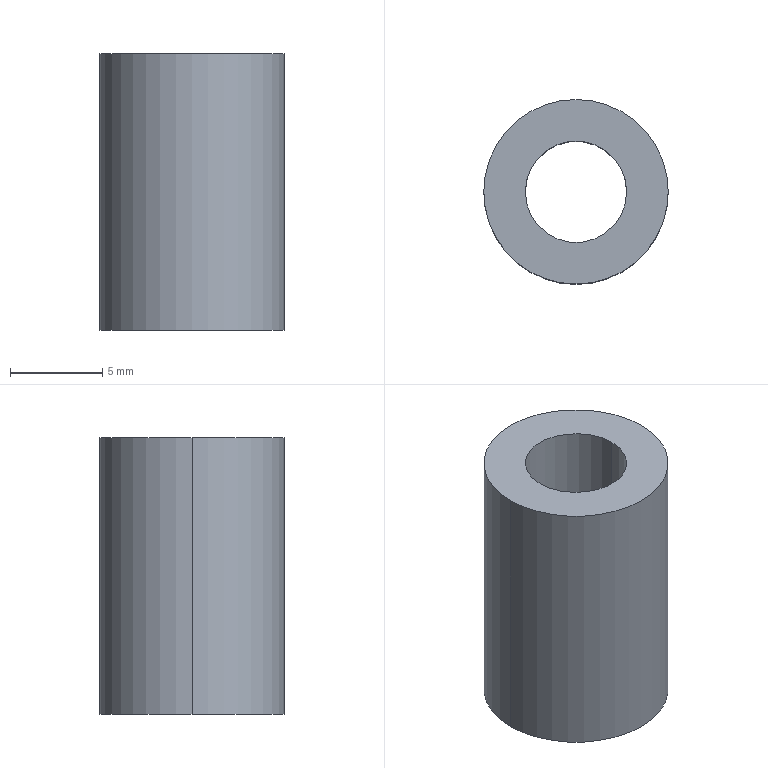Part | STEP file | positioning cylinder post | 1 solid | 6 faces | box 10 x 10 x 15 mm | volume 821.723 mm3 | cylinder 4 | plane 2 | commonest cylinder face diameters 5.5 x2 10 x2
STEP:
#1=CARTESIAN_POINT('',(0.,0.,0.));
#2=DIRECTION('',(0.,0.,1.));
#3=DIRECTION('',(1.,0.,0.));
#4=AXIS2_PLACEMENT_3D('',#1,#2,#3);
#5=CARTESIAN_POINT('',(-2.75,0.,15.));
#6=VERTEX_POINT('',#5);
#7=CARTESIAN_POINT('',(-2.75,0.,0.));
#8=VERTEX_POINT('',#7);
#9=CARTESIAN_POINT('',(-2.75,0.,15.));
#10=DIRECTION('',(0.,0.,-1.));
#11=VECTOR('',#10,1.);
#12=LINE('',#9,#11);
#13=CARTESIAN_POINT('',(0.,0.,15.));
#14=DIRECTION('',(0.,0.,-1.));
#15=DIRECTION('',(-1.,0.,0.));
#16=AXIS2_PLACEMENT_3D('',#13,#14,#15);
#17=CYLINDRICAL_SURFACE('',#16,2.75);
#18=CARTESIAN_POINT('',(6.283,0.));
#19=DIRECTION('',(0.,1.));
#20=VECTOR('',#19,1.);
#21=LINE('',#18,#20);
#22=(GEOMETRIC_REPRESENTATION_CONTEXT(2)PARAMETRIC_REPRESENTATION_CONTEXT()REPRESENTATION_CONTEXT('',''));
#23=DEFINITIONAL_REPRESENTATION('',(#21),#22);
#24=PCURVE('',#17,#23);
#25=CARTESIAN_POINT('',(0.,0.,15.));
#26=DIRECTION('',(0.,0.,-1.));
#27=DIRECTION('',(-1.,0.,0.));
#28=AXIS2_PLACEMENT_3D('',#25,#26,#27);
#29=CYLINDRICAL_SURFACE('',#28,2.75);
#30=CARTESIAN_POINT('',(0.,0.));
#31=DIRECTION('',(0.,1.));
#32=VECTOR('',#31,1.);
#33=LINE('',#30,#32);
#34=(GEOMETRIC_REPRESENTATION_CONTEXT(2)PARAMETRIC_REPRESENTATION_CONTEXT()REPRESENTATION_CONTEXT('',''));
#35=DEFINITIONAL_REPRESENTATION('',(#33),#34);
#36=PCURVE('',#29,#35);
#37=SURFACE_CURVE('',#12,(#24,#36),.PCURVE_S1.);
#38=EDGE_CURVE('',#6,#8,#37,.T.);
#39=ORIENTED_EDGE('',*,*,#38,.T.);
#40=CARTESIAN_POINT('',(2.75,0.,0.));
#41=VERTEX_POINT('',#40);
#42=CARTESIAN_POINT('',(0.,0.,0.));
#43=DIRECTION('',(0.,0.,1.));
#44=DIRECTION('',(1.,0.,0.));
#45=AXIS2_PLACEMENT_3D('',#42,#43,#44);
#46=CIRCLE('',#45,2.75);
#47=CARTESIAN_POINT('',(9.425,15.));
#48=DIRECTION('',(-1.,0.));
#49=VECTOR('',#48,1.);
#50=LINE('',#47,#49);
#51=(GEOMETRIC_REPRESENTATION_CONTEXT(2)PARAMETRIC_REPRESENTATION_CONTEXT()REPRESENTATION_CONTEXT('',''));
#52=DEFINITIONAL_REPRESENTATION('',(#50),#51);
#53=PCURVE('',#17,#52);
#54=CARTESIAN_POINT('',(0.,0.,0.));
#55=DIRECTION('',(0.,0.,1.));
#56=DIRECTION('',(1.,0.,0.));
#57=AXIS2_PLACEMENT_3D('',#54,#55,#56);
#58=PLANE('',#57);
#59=CARTESIAN_POINT('',(0.,0.));
#60=DIRECTION('',(1.,0.));
#61=AXIS2_PLACEMENT_2D('',#59,#60);
#62=CIRCLE('',#61,2.75);
#63=(GEOMETRIC_REPRESENTATION_CONTEXT(2)PARAMETRIC_REPRESENTATION_CONTEXT()REPRESENTATION_CONTEXT('',''));
#64=DEFINITIONAL_REPRESENTATION('',(#62),#63);
#65=PCURVE('',#58,#64);
#66=SURFACE_CURVE('',#46,(#53,#65),.PCURVE_S1.);
#67=EDGE_CURVE('',#8,#41,#66,.T.);
#68=ORIENTED_EDGE('',*,*,#67,.T.);
#69=CARTESIAN_POINT('',(2.75,0.,15.));
#70=VERTEX_POINT('',#69);
#71=CARTESIAN_POINT('',(2.75,0.,15.));
#72=DIRECTION('',(0.,0.,-1.));
#73=VECTOR('',#72,1.);
#74=LINE('',#71,#73);
#75=CARTESIAN_POINT('',(3.142,0.));
#76=DIRECTION('',(0.,1.));
#77=VECTOR('',#76,1.);
#78=LINE('',#75,#77);
#79=(GEOMETRIC_REPRESENTATION_CONTEXT(2)PARAMETRIC_REPRESENTATION_CONTEXT()REPRESENTATION_CONTEXT('',''));
#80=DEFINITIONAL_REPRESENTATION('',(#78),#79);
#81=PCURVE('',#17,#80);
#82=CARTESIAN_POINT('',(3.142,0.));
#83=DIRECTION('',(0.,1.));
#84=VECTOR('',#83,1.);
#85=LINE('',#82,#84);
#86=(GEOMETRIC_REPRESENTATION_CONTEXT(2)PARAMETRIC_REPRESENTATION_CONTEXT()REPRESENTATION_CONTEXT('',''));
#87=DEFINITIONAL_REPRESENTATION('',(#85),#86);
#88=PCURVE('',#29,#87);
#89=SURFACE_CURVE('',#74,(#81,#88),.PCURVE_S1.);
#90=EDGE_CURVE('',#70,#41,#89,.T.);
#91=ORIENTED_EDGE('',*,*,#90,.F.);
#92=CARTESIAN_POINT('',(0.,0.,15.));
#93=DIRECTION('',(0.,0.,1.));
#94=DIRECTION('',(1.,0.,0.));
#95=AXIS2_PLACEMENT_3D('',#92,#93,#94);
#96=CIRCLE('',#95,2.75);
#97=CARTESIAN_POINT('',(9.425,0.));
#98=DIRECTION('',(-1.,0.));
#99=VECTOR('',#98,1.);
#100=LINE('',#97,#99);
#101=(GEOMETRIC_REPRESENTATION_CONTEXT(2)PARAMETRIC_REPRESENTATION_CONTEXT()REPRESENTATION_CONTEXT('',''));
#102=DEFINITIONAL_REPRESENTATION('',(#100),#101);
#103=PCURVE('',#17,#102);
#104=CARTESIAN_POINT('',(0.,0.,15.));
#105=DIRECTION('',(0.,0.,1.));
#106=DIRECTION('',(1.,0.,0.));
#107=AXIS2_PLACEMENT_3D('',#104,#105,#106);
#108=PLANE('',#107);
#109=CARTESIAN_POINT('',(0.,0.));
#110=DIRECTION('',(1.,0.));
#111=AXIS2_PLACEMENT_2D('',#109,#110);
#112=CIRCLE('',#111,2.75);
#113=(GEOMETRIC_REPRESENTATION_CONTEXT(2)PARAMETRIC_REPRESENTATION_CONTEXT()REPRESENTATION_CONTEXT('',''));
#114=DEFINITIONAL_REPRESENTATION('',(#112),#113);
#115=PCURVE('',#108,#114);
#116=SURFACE_CURVE('',#96,(#103,#115),.PCURVE_S1.);
#117=EDGE_CURVE('',#6,#70,#116,.T.);
#118=ORIENTED_EDGE('',*,*,#117,.F.);
#119=EDGE_LOOP('',(#39,#68,#91,#118));
#120=FACE_BOUND('',#119,.F.);
#121=ADVANCED_FACE('',(#120),#17,.F.);
#122=CARTESIAN_POINT('',(5.,0.,15.));
#123=VERTEX_POINT('',#122);
#124=CARTESIAN_POINT('',(-5.,0.,15.));
#125=VERTEX_POINT('',#124);
#126=CARTESIAN_POINT('',(0.,0.,15.));
#127=DIRECTION('',(0.,0.,1.));
#128=DIRECTION('',(1.,0.,0.));
#129=AXIS2_PLACEMENT_3D('',#126,#127,#128);
#130=CIRCLE('',#129,5.);
#131=CARTESIAN_POINT('',(0.,0.,15.));
#132=DIRECTION('',(0.,0.,-1.));
#133=DIRECTION('',(-1.,0.,0.));
#134=AXIS2_PLACEMENT_3D('',#131,#132,#133);
#135=CYLINDRICAL_SURFACE('',#134,5.);
#136=CARTESIAN_POINT('',(3.142,0.));
#137=DIRECTION('',(-1.,0.));
#138=VECTOR('',#137,1.);
#139=LINE('',#136,#138);
#140=(GEOMETRIC_REPRESENTATION_CONTEXT(2)PARAMETRIC_REPRESENTATION_CONTEXT()REPRESENTATION_CONTEXT('',''));
#141=DEFINITIONAL_REPRESENTATION('',(#139),#140);
#142=PCURVE('',#135,#141);
#143=CARTESIAN_POINT('',(0.,0.));
#144=DIRECTION('',(1.,0.));
#145=AXIS2_PLACEMENT_2D('',#143,#144);
#146=CIRCLE('',#145,5.);
#147=(GEOMETRIC_REPRESENTATION_CONTEXT(2)PARAMETRIC_REPRESENTATION_CONTEXT()REPRESENTATION_CONTEXT('',''));
#148=DEFINITIONAL_REPRESENTATION('',(#146),#147);
#149=PCURVE('',#108,#148);
#150=SURFACE_CURVE('',#130,(#142,#149),.PCURVE_S1.);
#151=EDGE_CURVE('',#123,#125,#150,.T.);
#152=ORIENTED_EDGE('',*,*,#151,.F.);
#153=CARTESIAN_POINT('',(5.,0.,0.));
#154=VERTEX_POINT('',#153);
#155=CARTESIAN_POINT('',(5.,0.,15.));
#156=DIRECTION('',(0.,0.,-1.));
#157=VECTOR('',#156,1.);
#158=LINE('',#155,#157);
#159=CARTESIAN_POINT('',(3.142,0.));
#160=DIRECTION('',(0.,1.));
#161=VECTOR('',#160,1.);
#162=LINE('',#159,#161);
#163=(GEOMETRIC_REPRESENTATION_CONTEXT(2)PARAMETRIC_REPRESENTATION_CONTEXT()REPRESENTATION_CONTEXT('',''));
#164=DEFINITIONAL_REPRESENTATION('',(#162),#163);
#165=PCURVE('',#135,#164);
#166=CARTESIAN_POINT('',(0.,0.,15.));
#167=DIRECTION('',(0.,0.,-1.));
#168=DIRECTION('',(-1.,0.,0.));
#169=AXIS2_PLACEMENT_3D('',#166,#167,#168);
#170=CYLINDRICAL_SURFACE('',#169,5.);
#171=CARTESIAN_POINT('',(3.142,0.));
#172=DIRECTION('',(0.,1.));
#173=VECTOR('',#172,1.);
#174=LINE('',#171,#173);
#175=(GEOMETRIC_REPRESENTATION_CONTEXT(2)PARAMETRIC_REPRESENTATION_CONTEXT()REPRESENTATION_CONTEXT('',''));
#176=DEFINITIONAL_REPRESENTATION('',(#174),#175);
#177=PCURVE('',#170,#176);
#178=SURFACE_CURVE('',#158,(#165,#177),.PCURVE_S1.);
#179=EDGE_CURVE('',#123,#154,#178,.T.);
#180=ORIENTED_EDGE('',*,*,#179,.T.);
#181=CARTESIAN_POINT('',(-5.,0.,0.));
#182=VERTEX_POINT('',#181);
#183=CARTESIAN_POINT('',(0.,0.,0.));
#184=DIRECTION('',(0.,0.,1.));
#185=DIRECTION('',(1.,0.,0.));
#186=AXIS2_PLACEMENT_3D('',#183,#184,#185);
#187=CIRCLE('',#186,5.);
#188=CARTESIAN_POINT('',(3.142,15.));
#189=DIRECTION('',(-1.,0.));
#190=VECTOR('',#189,1.);
#191=LINE('',#188,#190);
#192=(GEOMETRIC_REPRESENTATION_CONTEXT(2)PARAMETRIC_REPRESENTATION_CONTEXT()REPRESENTATION_CONTEXT('',''));
#193=DEFINITIONAL_REPRESENTATION('',(#191),#192);
#194=PCURVE('',#135,#193);
#195=CARTESIAN_POINT('',(0.,0.));
#196=DIRECTION('',(1.,0.));
#197=AXIS2_PLACEMENT_2D('',#195,#196);
#198=CIRCLE('',#197,5.);
#199=(GEOMETRIC_REPRESENTATION_CONTEXT(2)PARAMETRIC_REPRESENTATION_CONTEXT()REPRESENTATION_CONTEXT('',''));
#200=DEFINITIONAL_REPRESENTATION('',(#198),#199);
#201=PCURVE('',#58,#200);
#202=SURFACE_CURVE('',#187,(#194,#201),.PCURVE_S1.);
#203=EDGE_CURVE('',#154,#182,#202,.T.);
#204=ORIENTED_EDGE('',*,*,#203,.T.);
#205=CARTESIAN_POINT('',(-5.,0.,15.));
#206=DIRECTION('',(0.,0.,-1.));
#207=VECTOR('',#206,1.);
#208=LINE('',#205,#207);
#209=CARTESIAN_POINT('',(0.,0.));
#210=DIRECTION('',(0.,1.));
#211=VECTOR('',#210,1.);
#212=LINE('',#209,#211);
#213=(GEOMETRIC_REPRESENTATION_CONTEXT(2)PARAMETRIC_REPRESENTATION_CONTEXT()REPRESENTATION_CONTEXT('',''));
#214=DEFINITIONAL_REPRESENTATION('',(#212),#213);
#215=PCURVE('',#135,#214);
#216=CARTESIAN_POINT('',(6.283,0.));
#217=DIRECTION('',(0.,1.));
#218=VECTOR('',#217,1.);
#219=LINE('',#216,#218);
#220=(GEOMETRIC_REPRESENTATION_CONTEXT(2)PARAMETRIC_REPRESENTATION_CONTEXT()REPRESENTATION_CONTEXT('',''));
#221=DEFINITIONAL_REPRESENTATION('',(#219),#220);
#222=PCURVE('',#170,#221);
#223=SURFACE_CURVE('',#208,(#215,#222),.PCURVE_S1.);
#224=EDGE_CURVE('',#125,#182,#223,.T.);
#225=ORIENTED_EDGE('',*,*,#224,.F.);
#226=EDGE_LOOP('',(#152,#180,#204,#225));
#227=FACE_BOUND('',#226,.T.);
#228=ADVANCED_FACE('',(#227),#135,.T.);
#229=CARTESIAN_POINT('',(0.,0.,15.));
#230=DIRECTION('',(0.,0.,1.));
#231=DIRECTION('',(1.,0.,0.));
#232=AXIS2_PLACEMENT_3D('',#229,#230,#231);
#233=CIRCLE('',#232,5.);
#234=CARTESIAN_POINT('',(0.,0.));
#235=DIRECTION('',(1.,0.));
#236=AXIS2_PLACEMENT_2D('',#234,#235);
#237=CIRCLE('',#236,5.);
#238=(GEOMETRIC_REPRESENTATION_CONTEXT(2)PARAMETRIC_REPRESENTATION_CONTEXT()REPRESENTATION_CONTEXT('',''));
#239=DEFINITIONAL_REPRESENTATION('',(#237),#238);
#240=PCURVE('',#108,#239);
#241=CARTESIAN_POINT('',(9.425,0.));
#242=DIRECTION('',(-1.,0.));
#243=VECTOR('',#242,1.);
#244=LINE('',#241,#243);
#245=(GEOMETRIC_REPRESENTATION_CONTEXT(2)PARAMETRIC_REPRESENTATION_CONTEXT()REPRESENTATION_CONTEXT('',''));
#246=DEFINITIONAL_REPRESENTATION('',(#244),#245);
#247=PCURVE('',#170,#246);
#248=SURFACE_CURVE('',#233,(#240,#247),.PCURVE_S1.);
#249=EDGE_CURVE('',#125,#123,#248,.T.);
#250=ORIENTED_EDGE('',*,*,#249,.T.);
#251=ORIENTED_EDGE('',*,*,#151,.T.);
#252=EDGE_LOOP('',(#250,#251));
#253=FACE_BOUND('',#252,.T.);
#254=ORIENTED_EDGE('',*,*,#117,.F.);
#255=CARTESIAN_POINT('',(0.,0.,15.));
#256=DIRECTION('',(0.,0.,1.));
#257=DIRECTION('',(1.,0.,0.));
#258=AXIS2_PLACEMENT_3D('',#255,#256,#257);
#259=CIRCLE('',#258,2.75);
#260=CARTESIAN_POINT('',(0.,0.));
#261=DIRECTION('',(1.,0.));
#262=AXIS2_PLACEMENT_2D('',#260,#261);
#263=CIRCLE('',#262,2.75);
#264=(GEOMETRIC_REPRESENTATION_CONTEXT(2)PARAMETRIC_REPRESENTATION_CONTEXT()REPRESENTATION_CONTEXT('',''));
#265=DEFINITIONAL_REPRESENTATION('',(#263),#264);
#266=PCURVE('',#108,#265);
#267=CARTESIAN_POINT('',(3.142,0.));
#268=DIRECTION('',(-1.,0.));
#269=VECTOR('',#268,1.);
#270=LINE('',#267,#269);
#271=(GEOMETRIC_REPRESENTATION_CONTEXT(2)PARAMETRIC_REPRESENTATION_CONTEXT()REPRESENTATION_CONTEXT('',''));
#272=DEFINITIONAL_REPRESENTATION('',(#270),#271);
#273=PCURVE('',#29,#272);
#274=SURFACE_CURVE('',#259,(#266,#273),.PCURVE_S1.);
#275=EDGE_CURVE('',#70,#6,#274,.T.);
#276=ORIENTED_EDGE('',*,*,#275,.F.);
#277=EDGE_LOOP('',(#254,#276));
#278=FACE_BOUND('',#277,.T.);
#279=ADVANCED_FACE('',(#253,#278),#108,.T.);
#280=CARTESIAN_POINT('',(0.,0.,0.));
#281=DIRECTION('',(0.,0.,1.));
#282=DIRECTION('',(1.,0.,0.));
#283=AXIS2_PLACEMENT_3D('',#280,#281,#282);
#284=CIRCLE('',#283,5.);
#285=CARTESIAN_POINT('',(0.,0.));
#286=DIRECTION('',(1.,0.));
#287=AXIS2_PLACEMENT_2D('',#285,#286);
#288=CIRCLE('',#287,5.);
#289=(GEOMETRIC_REPRESENTATION_CONTEXT(2)PARAMETRIC_REPRESENTATION_CONTEXT()REPRESENTATION_CONTEXT('',''));
#290=DEFINITIONAL_REPRESENTATION('',(#288),#289);
#291=PCURVE('',#58,#290);
#292=CARTESIAN_POINT('',(9.425,15.));
#293=DIRECTION('',(-1.,0.));
#294=VECTOR('',#293,1.);
#295=LINE('',#292,#294);
#296=(GEOMETRIC_REPRESENTATION_CONTEXT(2)PARAMETRIC_REPRESENTATION_CONTEXT()REPRESENTATION_CONTEXT('',''));
#297=DEFINITIONAL_REPRESENTATION('',(#295),#296);
#298=PCURVE('',#170,#297);
#299=SURFACE_CURVE('',#284,(#291,#298),.PCURVE_S1.);
#300=EDGE_CURVE('',#182,#154,#299,.T.);
#301=ORIENTED_EDGE('',*,*,#300,.F.);
#302=ORIENTED_EDGE('',*,*,#203,.F.);
#303=EDGE_LOOP('',(#301,#302));
#304=FACE_BOUND('',#303,.T.);
#305=ORIENTED_EDGE('',*,*,#67,.T.);
#306=CARTESIAN_POINT('',(0.,0.,0.));
#307=DIRECTION('',(0.,0.,1.));
#308=DIRECTION('',(1.,0.,0.));
#309=AXIS2_PLACEMENT_3D('',#306,#307,#308);
#310=CIRCLE('',#309,2.75);
#311=CARTESIAN_POINT('',(0.,0.));
#312=DIRECTION('',(1.,0.));
#313=AXIS2_PLACEMENT_2D('',#311,#312);
#314=CIRCLE('',#313,2.75);
#315=(GEOMETRIC_REPRESENTATION_CONTEXT(2)PARAMETRIC_REPRESENTATION_CONTEXT()REPRESENTATION_CONTEXT('',''));
#316=DEFINITIONAL_REPRESENTATION('',(#314),#315);
#317=PCURVE('',#58,#316);
#318=CARTESIAN_POINT('',(3.142,15.));
#319=DIRECTION('',(-1.,0.));
#320=VECTOR('',#319,1.);
#321=LINE('',#318,#320);
#322=(GEOMETRIC_REPRESENTATION_CONTEXT(2)PARAMETRIC_REPRESENTATION_CONTEXT()REPRESENTATION_CONTEXT('',''));
#323=DEFINITIONAL_REPRESENTATION('',(#321),#322);
#324=PCURVE('',#29,#323);
#325=SURFACE_CURVE('',#310,(#317,#324),.PCURVE_S1.);
#326=EDGE_CURVE('',#41,#8,#325,.T.);
#327=ORIENTED_EDGE('',*,*,#326,.T.);
#328=EDGE_LOOP('',(#305,#327));
#329=FACE_BOUND('',#328,.T.);
#330=ADVANCED_FACE('',(#304,#329),#58,.F.);
#331=ORIENTED_EDGE('',*,*,#179,.F.);
#332=ORIENTED_EDGE('',*,*,#249,.F.);
#333=ORIENTED_EDGE('',*,*,#224,.T.);
#334=ORIENTED_EDGE('',*,*,#300,.T.);
#335=EDGE_LOOP('',(#331,#332,#333,#334));
#336=FACE_BOUND('',#335,.T.);
#337=ADVANCED_FACE('',(#336),#170,.T.);
#338=ORIENTED_EDGE('',*,*,#326,.T.);
#339=ORIENTED_EDGE('',*,*,#38,.F.);
#340=ORIENTED_EDGE('',*,*,#275,.F.);
#341=ORIENTED_EDGE('',*,*,#90,.T.);
#342=EDGE_LOOP('',(#338,#339,#340,#341));
#343=FACE_BOUND('',#342,.F.);
#344=ADVANCED_FACE('',(#343),#29,.F.);
#345=CLOSED_SHELL('',(#121,#228,#279,#330,#337,#344));
#346=MANIFOLD_SOLID_BREP('',#345);
#347=(LENGTH_UNIT()NAMED_UNIT(*)SI_UNIT(.MILLI.,.METRE.));
#348=UNCERTAINTY_MEASURE_WITH_UNIT(LENGTH_MEASURE(0.0000001),#347,'','');
#349=(NAMED_UNIT(*)PLANE_ANGLE_UNIT()SI_UNIT($,.RADIAN.));
#350=(NAMED_UNIT(*)SI_UNIT($,.STERADIAN.)SOLID_ANGLE_UNIT());
#351=(GEOMETRIC_REPRESENTATION_CONTEXT(3)GLOBAL_UNCERTAINTY_ASSIGNED_CONTEXT((#348))GLOBAL_UNIT_ASSIGNED_CONTEXT((#347,#349,#350))REPRESENTATION_CONTEXT('',''));
#352=ADVANCED_BREP_SHAPE_REPRESENTATION('',(#4,#346),#351);